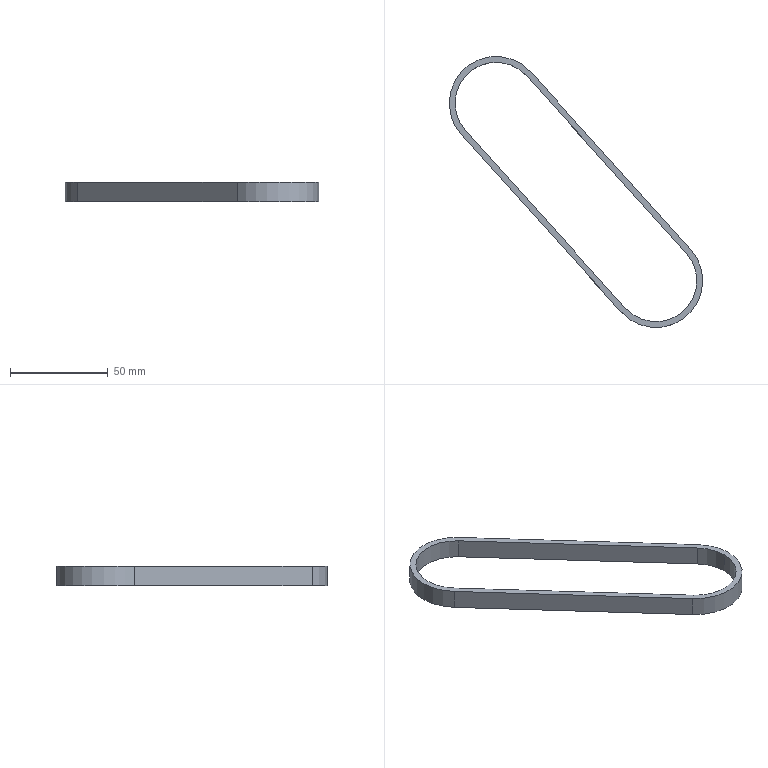Part | STEP file | 1 solid | 12 faces | box 130.012 x 138.996 x 10 mm | volume 11591 mm3 | plane 6 | cylinder 6 | commonest cylinder face diameters 42 x3 48 x3
STEP:
#1=CARTESIAN_POINT('',(0.,0.,0.));
#2=DIRECTION('',(0.,0.,1.));
#3=DIRECTION('',(1.,0.,0.));
#4=AXIS2_PLACEMENT_3D('',#1,#2,#3);
#5=CARTESIAN_POINT('',(-9.506,41.915,-2.));
#6=VERTEX_POINT('',#5);
#7=CARTESIAN_POINT('',(-91.518,132.912,-2.));
#8=VERTEX_POINT('',#7);
#9=CARTESIAN_POINT('',(15.599,14.059,-2.));
#10=DIRECTION('',(-0.6695,0.7428,0.));
#11=VECTOR('',#10,1.);
#12=LINE('',#9,#11);
#13=CARTESIAN_POINT('',(15.599,14.059,-12.));
#14=DIRECTION('',(0.7428,0.6695,0.));
#15=DIRECTION('',(0.,0.,-1.));
#16=AXIS2_PLACEMENT_3D('',#13,#14,#15);
#17=PLANE('',#16);
#18=CARTESIAN_POINT('',(-10.,0.));
#19=DIRECTION('',(0.,1.));
#20=VECTOR('',#19,1.);
#21=LINE('',#18,#20);
#22=(GEOMETRIC_REPRESENTATION_CONTEXT(2)PARAMETRIC_REPRESENTATION_CONTEXT()REPRESENTATION_CONTEXT('',''));
#23=DEFINITIONAL_REPRESENTATION('',(#21),#22);
#24=PCURVE('',#17,#23);
#25=CARTESIAN_POINT('',(0.,0.,-2.));
#26=DIRECTION('',(0.,0.,1.));
#27=DIRECTION('',(1.,0.,0.));
#28=AXIS2_PLACEMENT_3D('',#25,#26,#27);
#29=PLANE('',#28);
#30=CARTESIAN_POINT('',(15.599,14.059));
#31=DIRECTION('',(-0.6695,0.7428));
#32=VECTOR('',#31,1.);
#33=LINE('',#30,#32);
#34=(GEOMETRIC_REPRESENTATION_CONTEXT(2)PARAMETRIC_REPRESENTATION_CONTEXT()REPRESENTATION_CONTEXT('',''));
#35=DEFINITIONAL_REPRESENTATION('',(#33),#34);
#36=PCURVE('',#29,#35);
#37=SURFACE_CURVE('',#12,(#24,#36),.PCURVE_S1.);
#38=EDGE_CURVE('',#6,#8,#37,.T.);
#39=ORIENTED_EDGE('',*,*,#38,.T.);
#40=CARTESIAN_POINT('',(-91.518,132.912,-12.));
#41=VERTEX_POINT('',#40);
#42=CARTESIAN_POINT('',(-91.518,132.912,-12.));
#43=DIRECTION('',(0.,0.,1.));
#44=VECTOR('',#43,1.);
#45=LINE('',#42,#44);
#46=CARTESIAN_POINT('',(0.,160.));
#47=DIRECTION('',(-1.,0.));
#48=VECTOR('',#47,1.);
#49=LINE('',#46,#48);
#50=(GEOMETRIC_REPRESENTATION_CONTEXT(2)PARAMETRIC_REPRESENTATION_CONTEXT()REPRESENTATION_CONTEXT('',''));
#51=DEFINITIONAL_REPRESENTATION('',(#49),#50);
#52=PCURVE('',#17,#51);
#53=CARTESIAN_POINT('',(-107.117,118.852,-12.));
#54=DIRECTION('',(0.,0.,1.));
#55=DIRECTION('',(1.,0.,0.));
#56=AXIS2_PLACEMENT_3D('',#53,#54,#55);
#57=CYLINDRICAL_SURFACE('',#56,21.);
#58=CARTESIAN_POINT('',(0.7335,0.));
#59=DIRECTION('',(0.,1.));
#60=VECTOR('',#59,1.);
#61=LINE('',#58,#60);
#62=(GEOMETRIC_REPRESENTATION_CONTEXT(2)PARAMETRIC_REPRESENTATION_CONTEXT()REPRESENTATION_CONTEXT('',''));
#63=DEFINITIONAL_REPRESENTATION('',(#61),#62);
#64=PCURVE('',#57,#63);
#65=SURFACE_CURVE('',#45,(#52,#64),.PCURVE_S1.);
#66=EDGE_CURVE('',#41,#8,#65,.T.);
#67=ORIENTED_EDGE('',*,*,#66,.F.);
#68=CARTESIAN_POINT('',(-9.506,41.915,-12.));
#69=VERTEX_POINT('',#68);
#70=CARTESIAN_POINT('',(15.599,14.059,-12.));
#71=DIRECTION('',(-0.6695,0.7428,0.));
#72=VECTOR('',#71,1.);
#73=LINE('',#70,#72);
#74=CARTESIAN_POINT('',(0.,0.));
#75=DIRECTION('',(0.,1.));
#76=VECTOR('',#75,1.);
#77=LINE('',#74,#76);
#78=(GEOMETRIC_REPRESENTATION_CONTEXT(2)PARAMETRIC_REPRESENTATION_CONTEXT()REPRESENTATION_CONTEXT('',''));
#79=DEFINITIONAL_REPRESENTATION('',(#77),#78);
#80=PCURVE('',#17,#79);
#81=CARTESIAN_POINT('',(0.,0.,-12.));
#82=DIRECTION('',(0.,0.,1.));
#83=DIRECTION('',(1.,0.,0.));
#84=AXIS2_PLACEMENT_3D('',#81,#82,#83);
#85=PLANE('',#84);
#86=CARTESIAN_POINT('',(15.599,14.059));
#87=DIRECTION('',(-0.6695,0.7428));
#88=VECTOR('',#87,1.);
#89=LINE('',#86,#88);
#90=(GEOMETRIC_REPRESENTATION_CONTEXT(2)PARAMETRIC_REPRESENTATION_CONTEXT()REPRESENTATION_CONTEXT('',''));
#91=DEFINITIONAL_REPRESENTATION('',(#89),#90);
#92=PCURVE('',#85,#91);
#93=SURFACE_CURVE('',#73,(#80,#92),.PCURVE_S1.);
#94=EDGE_CURVE('',#69,#41,#93,.T.);
#95=ORIENTED_EDGE('',*,*,#94,.F.);
#96=CARTESIAN_POINT('',(-9.506,41.915,-12.));
#97=DIRECTION('',(0.,0.,1.));
#98=VECTOR('',#97,1.);
#99=LINE('',#96,#98);
#100=CARTESIAN_POINT('',(0.,37.5));
#101=DIRECTION('',(-1.,0.));
#102=VECTOR('',#101,1.);
#103=LINE('',#100,#102);
#104=(GEOMETRIC_REPRESENTATION_CONTEXT(2)PARAMETRIC_REPRESENTATION_CONTEXT()REPRESENTATION_CONTEXT('',''));
#105=DEFINITIONAL_REPRESENTATION('',(#103),#104);
#106=PCURVE('',#17,#105);
#107=CARTESIAN_POINT('',(-25.106,27.856,-12.));
#108=DIRECTION('',(0.,0.,1.));
#109=DIRECTION('',(1.,0.,0.));
#110=AXIS2_PLACEMENT_3D('',#107,#108,#109);
#111=CYLINDRICAL_SURFACE('',#110,21.);
#112=CARTESIAN_POINT('',(0.7335,0.));
#113=DIRECTION('',(0.,1.));
#114=VECTOR('',#113,1.);
#115=LINE('',#112,#114);
#116=(GEOMETRIC_REPRESENTATION_CONTEXT(2)PARAMETRIC_REPRESENTATION_CONTEXT()REPRESENTATION_CONTEXT('',''));
#117=DEFINITIONAL_REPRESENTATION('',(#115),#116);
#118=PCURVE('',#111,#117);
#119=SURFACE_CURVE('',#99,(#106,#118),.PCURVE_S1.);
#120=EDGE_CURVE('',#69,#6,#119,.T.);
#121=ORIENTED_EDGE('',*,*,#120,.T.);
#122=EDGE_LOOP('',(#39,#67,#95,#121));
#123=FACE_BOUND('',#122,.T.);
#124=ADVANCED_FACE('',(#123),#17,.F.);
#125=ORIENTED_EDGE('',*,*,#66,.F.);
#126=CARTESIAN_POINT('',(-122.717,104.793,-12.));
#127=VERTEX_POINT('',#126);
#128=CARTESIAN_POINT('',(-107.117,118.852,-12.));
#129=DIRECTION('',(0.,0.,1.));
#130=DIRECTION('',(1.,0.,0.));
#131=AXIS2_PLACEMENT_3D('',#128,#129,#130);
#132=CIRCLE('',#131,21.);
#133=CARTESIAN_POINT('',(0.,0.));
#134=DIRECTION('',(1.,0.));
#135=VECTOR('',#134,1.);
#136=LINE('',#133,#135);
#137=(GEOMETRIC_REPRESENTATION_CONTEXT(2)PARAMETRIC_REPRESENTATION_CONTEXT()REPRESENTATION_CONTEXT('',''));
#138=DEFINITIONAL_REPRESENTATION('',(#136),#137);
#139=PCURVE('',#57,#138);
#140=CARTESIAN_POINT('',(-107.117,118.852));
#141=DIRECTION('',(1.,0.));
#142=AXIS2_PLACEMENT_2D('',#140,#141);
#143=CIRCLE('',#142,21.);
#144=(GEOMETRIC_REPRESENTATION_CONTEXT(2)PARAMETRIC_REPRESENTATION_CONTEXT()REPRESENTATION_CONTEXT('',''));
#145=DEFINITIONAL_REPRESENTATION('',(#143),#144);
#146=PCURVE('',#85,#145);
#147=SURFACE_CURVE('',#132,(#139,#146),.PCURVE_S1.);
#148=EDGE_CURVE('',#41,#127,#147,.T.);
#149=ORIENTED_EDGE('',*,*,#148,.T.);
#150=CARTESIAN_POINT('',(-122.717,104.793,-2.));
#151=VERTEX_POINT('',#150);
#152=CARTESIAN_POINT('',(-122.717,104.793,-12.));
#153=DIRECTION('',(0.,0.,1.));
#154=VECTOR('',#153,1.);
#155=LINE('',#152,#154);
#156=CARTESIAN_POINT('',(3.875,0.));
#157=DIRECTION('',(0.,1.));
#158=VECTOR('',#157,1.);
#159=LINE('',#156,#158);
#160=(GEOMETRIC_REPRESENTATION_CONTEXT(2)PARAMETRIC_REPRESENTATION_CONTEXT()REPRESENTATION_CONTEXT('',''));
#161=DEFINITIONAL_REPRESENTATION('',(#159),#160);
#162=PCURVE('',#57,#161);
#163=CARTESIAN_POINT('',(-15.599,-14.059,-12.));
#164=DIRECTION('',(-0.7428,-0.6695,0.));
#165=DIRECTION('',(-0.6695,0.7428,0.));
#166=AXIS2_PLACEMENT_3D('',#163,#164,#165);
#167=PLANE('',#166);
#168=CARTESIAN_POINT('',(160.,0.));
#169=DIRECTION('',(0.,-1.));
#170=VECTOR('',#169,1.);
#171=LINE('',#168,#170);
#172=(GEOMETRIC_REPRESENTATION_CONTEXT(2)PARAMETRIC_REPRESENTATION_CONTEXT()REPRESENTATION_CONTEXT('',''));
#173=DEFINITIONAL_REPRESENTATION('',(#171),#172);
#174=PCURVE('',#167,#173);
#175=SURFACE_CURVE('',#155,(#162,#174),.PCURVE_S1.);
#176=EDGE_CURVE('',#127,#151,#175,.T.);
#177=ORIENTED_EDGE('',*,*,#176,.T.);
#178=CARTESIAN_POINT('',(-107.117,118.852,-2.));
#179=DIRECTION('',(0.,0.,1.));
#180=DIRECTION('',(1.,0.,0.));
#181=AXIS2_PLACEMENT_3D('',#178,#179,#180);
#182=CIRCLE('',#181,21.);
#183=CARTESIAN_POINT('',(0.,10.));
#184=DIRECTION('',(1.,0.));
#185=VECTOR('',#184,1.);
#186=LINE('',#183,#185);
#187=(GEOMETRIC_REPRESENTATION_CONTEXT(2)PARAMETRIC_REPRESENTATION_CONTEXT()REPRESENTATION_CONTEXT('',''));
#188=DEFINITIONAL_REPRESENTATION('',(#186),#187);
#189=PCURVE('',#57,#188);
#190=CARTESIAN_POINT('',(-107.117,118.852));
#191=DIRECTION('',(1.,0.));
#192=AXIS2_PLACEMENT_2D('',#190,#191);
#193=CIRCLE('',#192,21.);
#194=(GEOMETRIC_REPRESENTATION_CONTEXT(2)PARAMETRIC_REPRESENTATION_CONTEXT()REPRESENTATION_CONTEXT('',''));
#195=DEFINITIONAL_REPRESENTATION('',(#193),#194);
#196=PCURVE('',#29,#195);
#197=SURFACE_CURVE('',#182,(#189,#196),.PCURVE_S1.);
#198=EDGE_CURVE('',#8,#151,#197,.T.);
#199=ORIENTED_EDGE('',*,*,#198,.F.);
#200=EDGE_LOOP('',(#125,#149,#177,#199));
#201=FACE_BOUND('',#200,.F.);
#202=ADVANCED_FACE('',(#201),#57,.F.);
#203=CARTESIAN_POINT('',(-40.705,13.797,-2.));
#204=VERTEX_POINT('',#203);
#205=CARTESIAN_POINT('',(-15.599,-14.059,-2.));
#206=DIRECTION('',(0.6695,-0.7428,0.));
#207=VECTOR('',#206,1.);
#208=LINE('',#205,#207);
#209=CARTESIAN_POINT('',(0.,-10.));
#210=DIRECTION('',(-1.,0.));
#211=VECTOR('',#210,1.);
#212=LINE('',#209,#211);
#213=(GEOMETRIC_REPRESENTATION_CONTEXT(2)PARAMETRIC_REPRESENTATION_CONTEXT()REPRESENTATION_CONTEXT('',''));
#214=DEFINITIONAL_REPRESENTATION('',(#212),#213);
#215=PCURVE('',#167,#214);
#216=CARTESIAN_POINT('',(-15.599,-14.059));
#217=DIRECTION('',(0.6695,-0.7428));
#218=VECTOR('',#217,1.);
#219=LINE('',#216,#218);
#220=(GEOMETRIC_REPRESENTATION_CONTEXT(2)PARAMETRIC_REPRESENTATION_CONTEXT()REPRESENTATION_CONTEXT('',''));
#221=DEFINITIONAL_REPRESENTATION('',(#219),#220);
#222=PCURVE('',#29,#221);
#223=SURFACE_CURVE('',#208,(#215,#222),.PCURVE_S1.);
#224=EDGE_CURVE('',#151,#204,#223,.T.);
#225=ORIENTED_EDGE('',*,*,#224,.T.);
#226=CARTESIAN_POINT('',(-40.705,13.797,-12.));
#227=VERTEX_POINT('',#226);
#228=CARTESIAN_POINT('',(-40.705,13.797,-12.));
#229=DIRECTION('',(0.,0.,1.));
#230=VECTOR('',#229,1.);
#231=LINE('',#228,#230);
#232=CARTESIAN_POINT('',(37.5,0.));
#233=DIRECTION('',(0.,-1.));
#234=VECTOR('',#233,1.);
#235=LINE('',#232,#234);
#236=(GEOMETRIC_REPRESENTATION_CONTEXT(2)PARAMETRIC_REPRESENTATION_CONTEXT()REPRESENTATION_CONTEXT('',''));
#237=DEFINITIONAL_REPRESENTATION('',(#235),#236);
#238=PCURVE('',#167,#237);
#239=CARTESIAN_POINT('',(-25.106,27.856,-12.));
#240=DIRECTION('',(0.,0.,1.));
#241=DIRECTION('',(1.,0.,0.));
#242=AXIS2_PLACEMENT_3D('',#239,#240,#241);
#243=CYLINDRICAL_SURFACE('',#242,21.);
#244=CARTESIAN_POINT('',(3.875,0.));
#245=DIRECTION('',(0.,1.));
#246=VECTOR('',#245,1.);
#247=LINE('',#244,#246);
#248=(GEOMETRIC_REPRESENTATION_CONTEXT(2)PARAMETRIC_REPRESENTATION_CONTEXT()REPRESENTATION_CONTEXT('',''));
#249=DEFINITIONAL_REPRESENTATION('',(#247),#248);
#250=PCURVE('',#243,#249);
#251=SURFACE_CURVE('',#231,(#238,#250),.PCURVE_S1.);
#252=EDGE_CURVE('',#227,#204,#251,.T.);
#253=ORIENTED_EDGE('',*,*,#252,.F.);
#254=CARTESIAN_POINT('',(-15.599,-14.059,-12.));
#255=DIRECTION('',(0.6695,-0.7428,0.));
#256=VECTOR('',#255,1.);
#257=LINE('',#254,#256);
#258=CARTESIAN_POINT('',(0.,0.));
#259=DIRECTION('',(-1.,0.));
#260=VECTOR('',#259,1.);
#261=LINE('',#258,#260);
#262=(GEOMETRIC_REPRESENTATION_CONTEXT(2)PARAMETRIC_REPRESENTATION_CONTEXT()REPRESENTATION_CONTEXT('',''));
#263=DEFINITIONAL_REPRESENTATION('',(#261),#262);
#264=PCURVE('',#167,#263);
#265=CARTESIAN_POINT('',(-15.599,-14.059));
#266=DIRECTION('',(0.6695,-0.7428));
#267=VECTOR('',#266,1.);
#268=LINE('',#265,#267);
#269=(GEOMETRIC_REPRESENTATION_CONTEXT(2)PARAMETRIC_REPRESENTATION_CONTEXT()REPRESENTATION_CONTEXT('',''));
#270=DEFINITIONAL_REPRESENTATION('',(#268),#269);
#271=PCURVE('',#85,#270);
#272=SURFACE_CURVE('',#257,(#264,#271),.PCURVE_S1.);
#273=EDGE_CURVE('',#127,#227,#272,.T.);
#274=ORIENTED_EDGE('',*,*,#273,.F.);
#275=ORIENTED_EDGE('',*,*,#176,.T.);
#276=EDGE_LOOP('',(#225,#253,#274,#275));
#277=FACE_BOUND('',#276,.T.);
#278=ADVANCED_FACE('',(#277),#167,.F.);
#279=CARTESIAN_POINT('',(-4.106,27.856,-2.));
#280=VERTEX_POINT('',#279);
#281=CARTESIAN_POINT('',(-25.106,27.856,-2.));
#282=DIRECTION('',(0.,0.,1.));
#283=DIRECTION('',(1.,0.,0.));
#284=AXIS2_PLACEMENT_3D('',#281,#282,#283);
#285=CIRCLE('',#284,21.);
#286=CARTESIAN_POINT('',(0.,10.));
#287=DIRECTION('',(1.,0.));
#288=VECTOR('',#287,1.);
#289=LINE('',#286,#288);
#290=(GEOMETRIC_REPRESENTATION_CONTEXT(2)PARAMETRIC_REPRESENTATION_CONTEXT()REPRESENTATION_CONTEXT('',''));
#291=DEFINITIONAL_REPRESENTATION('',(#289),#290);
#292=PCURVE('',#243,#291);
#293=CARTESIAN_POINT('',(-25.106,27.856));
#294=DIRECTION('',(1.,0.));
#295=AXIS2_PLACEMENT_2D('',#293,#294);
#296=CIRCLE('',#295,21.);
#297=(GEOMETRIC_REPRESENTATION_CONTEXT(2)PARAMETRIC_REPRESENTATION_CONTEXT()REPRESENTATION_CONTEXT('',''));
#298=DEFINITIONAL_REPRESENTATION('',(#296),#297);
#299=PCURVE('',#29,#298);
#300=SURFACE_CURVE('',#285,(#292,#299),.PCURVE_S1.);
#301=EDGE_CURVE('',#204,#280,#300,.T.);
#302=ORIENTED_EDGE('',*,*,#301,.F.);
#303=ORIENTED_EDGE('',*,*,#252,.F.);
#304=CARTESIAN_POINT('',(-4.106,27.856,-12.));
#305=VERTEX_POINT('',#304);
#306=CARTESIAN_POINT('',(-25.106,27.856,-12.));
#307=DIRECTION('',(0.,0.,1.));
#308=DIRECTION('',(1.,0.,0.));
#309=AXIS2_PLACEMENT_3D('',#306,#307,#308);
#310=CIRCLE('',#309,21.);
#311=CARTESIAN_POINT('',(0.,0.));
#312=DIRECTION('',(1.,0.));
#313=VECTOR('',#312,1.);
#314=LINE('',#311,#313);
#315=(GEOMETRIC_REPRESENTATION_CONTEXT(2)PARAMETRIC_REPRESENTATION_CONTEXT()REPRESENTATION_CONTEXT('',''));
#316=DEFINITIONAL_REPRESENTATION('',(#314),#315);
#317=PCURVE('',#243,#316);
#318=CARTESIAN_POINT('',(-25.106,27.856));
#319=DIRECTION('',(1.,0.));
#320=AXIS2_PLACEMENT_2D('',#318,#319);
#321=CIRCLE('',#320,21.);
#322=(GEOMETRIC_REPRESENTATION_CONTEXT(2)PARAMETRIC_REPRESENTATION_CONTEXT()REPRESENTATION_CONTEXT('',''));
#323=DEFINITIONAL_REPRESENTATION('',(#321),#322);
#324=PCURVE('',#85,#323);
#325=SURFACE_CURVE('',#310,(#317,#324),.PCURVE_S1.);
#326=EDGE_CURVE('',#227,#305,#325,.T.);
#327=ORIENTED_EDGE('',*,*,#326,.T.);
#328=CARTESIAN_POINT('',(-4.106,27.856,-12.));
#329=DIRECTION('',(0.,0.,1.));
#330=VECTOR('',#329,1.);
#331=LINE('',#328,#330);
#332=CARTESIAN_POINT('',(6.283,0.));
#333=DIRECTION('',(0.,1.));
#334=VECTOR('',#333,1.);
#335=LINE('',#332,#334);
#336=(GEOMETRIC_REPRESENTATION_CONTEXT(2)PARAMETRIC_REPRESENTATION_CONTEXT()REPRESENTATION_CONTEXT('',''));
#337=DEFINITIONAL_REPRESENTATION('',(#335),#336);
#338=PCURVE('',#243,#337);
#339=CARTESIAN_POINT('',(0.,0.));
#340=DIRECTION('',(0.,1.));
#341=VECTOR('',#340,1.);
#342=LINE('',#339,#341);
#343=(GEOMETRIC_REPRESENTATION_CONTEXT(2)PARAMETRIC_REPRESENTATION_CONTEXT()REPRESENTATION_CONTEXT('',''));
#344=DEFINITIONAL_REPRESENTATION('',(#342),#343);
#345=PCURVE('',#111,#344);
#346=SURFACE_CURVE('',#331,(#338,#345),.PCURVE_S1.);
#347=EDGE_CURVE('',#305,#280,#346,.T.);
#348=ORIENTED_EDGE('',*,*,#347,.T.);
#349=EDGE_LOOP('',(#302,#303,#327,#348));
#350=FACE_BOUND('',#349,.F.);
#351=ADVANCED_FACE('',(#350),#243,.F.);
#352=ORIENTED_EDGE('',*,*,#301,.F.);
#353=ORIENTED_EDGE('',*,*,#224,.F.);
#354=ORIENTED_EDGE('',*,*,#198,.F.);
#355=ORIENTED_EDGE('',*,*,#38,.F.);
#356=CARTESIAN_POINT('',(-25.106,27.856,-2.));
#357=DIRECTION('',(0.,0.,1.));
#358=DIRECTION('',(1.,0.,0.));
#359=AXIS2_PLACEMENT_3D('',#356,#357,#358);
#360=CIRCLE('',#359,21.);
#361=CARTESIAN_POINT('',(-25.106,27.856));
#362=DIRECTION('',(1.,0.));
#363=AXIS2_PLACEMENT_2D('',#361,#362);
#364=CIRCLE('',#363,21.);
#365=(GEOMETRIC_REPRESENTATION_CONTEXT(2)PARAMETRIC_REPRESENTATION_CONTEXT()REPRESENTATION_CONTEXT('',''));
#366=DEFINITIONAL_REPRESENTATION('',(#364),#365);
#367=PCURVE('',#29,#366);
#368=CARTESIAN_POINT('',(0.,10.));
#369=DIRECTION('',(1.,0.));
#370=VECTOR('',#369,1.);
#371=LINE('',#368,#370);
#372=(GEOMETRIC_REPRESENTATION_CONTEXT(2)PARAMETRIC_REPRESENTATION_CONTEXT()REPRESENTATION_CONTEXT('',''));
#373=DEFINITIONAL_REPRESENTATION('',(#371),#372);
#374=PCURVE('',#111,#373);
#375=SURFACE_CURVE('',#360,(#367,#374),.PCURVE_S1.);
#376=EDGE_CURVE('',#280,#6,#375,.T.);
#377=ORIENTED_EDGE('',*,*,#376,.F.);
#378=EDGE_LOOP('',(#352,#353,#354,#355,#377));
#379=FACE_BOUND('',#378,.T.);
#380=CARTESIAN_POINT('',(-42.933,11.788,-2.));
#381=VERTEX_POINT('',#380);
#382=CARTESIAN_POINT('',(-1.106,27.856,-2.));
#383=VERTEX_POINT('',#382);
#384=CARTESIAN_POINT('',(-25.106,27.856,-2.));
#385=DIRECTION('',(0.,0.,1.));
#386=DIRECTION('',(1.,0.,0.));
#387=AXIS2_PLACEMENT_3D('',#384,#385,#386);
#388=CIRCLE('',#387,24.);
#389=CARTESIAN_POINT('',(-25.106,27.856));
#390=DIRECTION('',(1.,0.));
#391=AXIS2_PLACEMENT_2D('',#389,#390);
#392=CIRCLE('',#391,24.);
#393=(GEOMETRIC_REPRESENTATION_CONTEXT(2)PARAMETRIC_REPRESENTATION_CONTEXT()REPRESENTATION_CONTEXT('',''));
#394=DEFINITIONAL_REPRESENTATION('',(#392),#393);
#395=PCURVE('',#29,#394);
#396=CARTESIAN_POINT('',(-25.106,27.856,-12.));
#397=DIRECTION('',(0.,0.,1.));
#398=DIRECTION('',(1.,0.,0.));
#399=AXIS2_PLACEMENT_3D('',#396,#397,#398);
#400=CYLINDRICAL_SURFACE('',#399,24.);
#401=CARTESIAN_POINT('',(0.,10.));
#402=DIRECTION('',(1.,0.));
#403=VECTOR('',#402,1.);
#404=LINE('',#401,#403);
#405=(GEOMETRIC_REPRESENTATION_CONTEXT(2)PARAMETRIC_REPRESENTATION_CONTEXT()REPRESENTATION_CONTEXT('',''));
#406=DEFINITIONAL_REPRESENTATION('',(#404),#405);
#407=PCURVE('',#400,#406);
#408=SURFACE_CURVE('',#388,(#395,#407),.PCURVE_S1.);
#409=EDGE_CURVE('',#381,#383,#408,.T.);
#410=ORIENTED_EDGE('',*,*,#409,.T.);
#411=CARTESIAN_POINT('',(-7.278,43.924,-2.));
#412=VERTEX_POINT('',#411);
#413=CARTESIAN_POINT('',(-25.106,27.856,-2.));
#414=DIRECTION('',(0.,0.,1.));
#415=DIRECTION('',(1.,0.,0.));
#416=AXIS2_PLACEMENT_3D('',#413,#414,#415);
#417=CIRCLE('',#416,24.);
#418=CARTESIAN_POINT('',(-25.106,27.856));
#419=DIRECTION('',(1.,0.));
#420=AXIS2_PLACEMENT_2D('',#418,#419);
#421=CIRCLE('',#420,24.);
#422=(GEOMETRIC_REPRESENTATION_CONTEXT(2)PARAMETRIC_REPRESENTATION_CONTEXT()REPRESENTATION_CONTEXT('',''));
#423=DEFINITIONAL_REPRESENTATION('',(#421),#422);
#424=PCURVE('',#29,#423);
#425=CARTESIAN_POINT('',(-25.106,27.856,-12.));
#426=DIRECTION('',(0.,0.,1.));
#427=DIRECTION('',(1.,0.,0.));
#428=AXIS2_PLACEMENT_3D('',#425,#426,#427);
#429=CYLINDRICAL_SURFACE('',#428,24.);
#430=CARTESIAN_POINT('',(0.,10.));
#431=DIRECTION('',(1.,0.));
#432=VECTOR('',#431,1.);
#433=LINE('',#430,#432);
#434=(GEOMETRIC_REPRESENTATION_CONTEXT(2)PARAMETRIC_REPRESENTATION_CONTEXT()REPRESENTATION_CONTEXT('',''));
#435=DEFINITIONAL_REPRESENTATION('',(#433),#434);
#436=PCURVE('',#429,#435);
#437=SURFACE_CURVE('',#417,(#424,#436),.PCURVE_S1.);
#438=EDGE_CURVE('',#383,#412,#437,.T.);
#439=ORIENTED_EDGE('',*,*,#438,.T.);
#440=CARTESIAN_POINT('',(-89.289,134.92,-2.));
#441=VERTEX_POINT('',#440);
#442=CARTESIAN_POINT('',(17.828,16.068,-2.));
#443=DIRECTION('',(-0.6695,0.7428,0.));
#444=VECTOR('',#443,1.);
#445=LINE('',#442,#444);
#446=CARTESIAN_POINT('',(17.828,16.068));
#447=DIRECTION('',(-0.6695,0.7428));
#448=VECTOR('',#447,1.);
#449=LINE('',#446,#448);
#450=(GEOMETRIC_REPRESENTATION_CONTEXT(2)PARAMETRIC_REPRESENTATION_CONTEXT()REPRESENTATION_CONTEXT('',''));
#451=DEFINITIONAL_REPRESENTATION('',(#449),#450);
#452=PCURVE('',#29,#451);
#453=CARTESIAN_POINT('',(17.828,16.068,-12.));
#454=DIRECTION('',(0.7428,0.6695,0.));
#455=DIRECTION('',(0.,0.,-1.));
#456=AXIS2_PLACEMENT_3D('',#453,#454,#455);
#457=PLANE('',#456);
#458=CARTESIAN_POINT('',(-10.,0.));
#459=DIRECTION('',(0.,1.));
#460=VECTOR('',#459,1.);
#461=LINE('',#458,#460);
#462=(GEOMETRIC_REPRESENTATION_CONTEXT(2)PARAMETRIC_REPRESENTATION_CONTEXT()REPRESENTATION_CONTEXT('',''));
#463=DEFINITIONAL_REPRESENTATION('',(#461),#462);
#464=PCURVE('',#457,#463);
#465=SURFACE_CURVE('',#445,(#452,#464),.PCURVE_S1.);
#466=EDGE_CURVE('',#412,#441,#465,.T.);
#467=ORIENTED_EDGE('',*,*,#466,.T.);
#468=CARTESIAN_POINT('',(-124.945,102.785,-2.));
#469=VERTEX_POINT('',#468);
#470=CARTESIAN_POINT('',(-107.117,118.852,-2.));
#471=DIRECTION('',(0.,0.,1.));
#472=DIRECTION('',(1.,0.,0.));
#473=AXIS2_PLACEMENT_3D('',#470,#471,#472);
#474=CIRCLE('',#473,24.);
#475=CARTESIAN_POINT('',(-107.117,118.852));
#476=DIRECTION('',(1.,0.));
#477=AXIS2_PLACEMENT_2D('',#475,#476);
#478=CIRCLE('',#477,24.);
#479=(GEOMETRIC_REPRESENTATION_CONTEXT(2)PARAMETRIC_REPRESENTATION_CONTEXT()REPRESENTATION_CONTEXT('',''));
#480=DEFINITIONAL_REPRESENTATION('',(#478),#479);
#481=PCURVE('',#29,#480);
#482=CARTESIAN_POINT('',(-107.117,118.852,-12.));
#483=DIRECTION('',(0.,0.,1.));
#484=DIRECTION('',(1.,0.,0.));
#485=AXIS2_PLACEMENT_3D('',#482,#483,#484);
#486=CYLINDRICAL_SURFACE('',#485,24.);
#487=CARTESIAN_POINT('',(0.,10.));
#488=DIRECTION('',(1.,0.));
#489=VECTOR('',#488,1.);
#490=LINE('',#487,#489);
#491=(GEOMETRIC_REPRESENTATION_CONTEXT(2)PARAMETRIC_REPRESENTATION_CONTEXT()REPRESENTATION_CONTEXT('',''));
#492=DEFINITIONAL_REPRESENTATION('',(#490),#491);
#493=PCURVE('',#486,#492);
#494=SURFACE_CURVE('',#474,(#481,#493),.PCURVE_S1.);
#495=EDGE_CURVE('',#441,#469,#494,.T.);
#496=ORIENTED_EDGE('',*,*,#495,.T.);
#497=CARTESIAN_POINT('',(-17.828,-16.068,-2.));
#498=DIRECTION('',(0.6695,-0.7428,0.));
#499=VECTOR('',#498,1.);
#500=LINE('',#497,#499);
#501=CARTESIAN_POINT('',(-17.828,-16.068));
#502=DIRECTION('',(0.6695,-0.7428));
#503=VECTOR('',#502,1.);
#504=LINE('',#501,#503);
#505=(GEOMETRIC_REPRESENTATION_CONTEXT(2)PARAMETRIC_REPRESENTATION_CONTEXT()REPRESENTATION_CONTEXT('',''));
#506=DEFINITIONAL_REPRESENTATION('',(#504),#505);
#507=PCURVE('',#29,#506);
#508=CARTESIAN_POINT('',(-17.828,-16.068,-12.));
#509=DIRECTION('',(-0.7428,-0.6695,0.));
#510=DIRECTION('',(-0.6695,0.7428,0.));
#511=AXIS2_PLACEMENT_3D('',#508,#509,#510);
#512=PLANE('',#511);
#513=CARTESIAN_POINT('',(0.,-10.));
#514=DIRECTION('',(-1.,0.));
#515=VECTOR('',#514,1.);
#516=LINE('',#513,#515);
#517=(GEOMETRIC_REPRESENTATION_CONTEXT(2)PARAMETRIC_REPRESENTATION_CONTEXT()REPRESENTATION_CONTEXT('',''));
#518=DEFINITIONAL_REPRESENTATION('',(#516),#517);
#519=PCURVE('',#512,#518);
#520=SURFACE_CURVE('',#500,(#507,#519),.PCURVE_S1.);
#521=EDGE_CURVE('',#469,#381,#520,.T.);
#522=ORIENTED_EDGE('',*,*,#521,.T.);
#523=EDGE_LOOP('',(#410,#439,#467,#496,#522));
#524=FACE_BOUND('',#523,.T.);
#525=ADVANCED_FACE('',(#379,#524),#29,.T.);
#526=ORIENTED_EDGE('',*,*,#273,.T.);
#527=ORIENTED_EDGE('',*,*,#326,.T.);
#528=CARTESIAN_POINT('',(-25.106,27.856,-12.));
#529=DIRECTION('',(0.,0.,1.));
#530=DIRECTION('',(1.,0.,0.));
#531=AXIS2_PLACEMENT_3D('',#528,#529,#530);
#532=CIRCLE('',#531,21.);
#533=CARTESIAN_POINT('',(-25.106,27.856));
#534=DIRECTION('',(1.,0.));
#535=AXIS2_PLACEMENT_2D('',#533,#534);
#536=CIRCLE('',#535,21.);
#537=(GEOMETRIC_REPRESENTATION_CONTEXT(2)PARAMETRIC_REPRESENTATION_CONTEXT()REPRESENTATION_CONTEXT('',''));
#538=DEFINITIONAL_REPRESENTATION('',(#536),#537);
#539=PCURVE('',#85,#538);
#540=CARTESIAN_POINT('',(0.,0.));
#541=DIRECTION('',(1.,0.));
#542=VECTOR('',#541,1.);
#543=LINE('',#540,#542);
#544=(GEOMETRIC_REPRESENTATION_CONTEXT(2)PARAMETRIC_REPRESENTATION_CONTEXT()REPRESENTATION_CONTEXT('',''));
#545=DEFINITIONAL_REPRESENTATION('',(#543),#544);
#546=PCURVE('',#111,#545);
#547=SURFACE_CURVE('',#532,(#539,#546),.PCURVE_S1.);
#548=EDGE_CURVE('',#305,#69,#547,.T.);
#549=ORIENTED_EDGE('',*,*,#548,.T.);
#550=ORIENTED_EDGE('',*,*,#94,.T.);
#551=ORIENTED_EDGE('',*,*,#148,.T.);
#552=EDGE_LOOP('',(#526,#527,#549,#550,#551));
#553=FACE_BOUND('',#552,.T.);
#554=CARTESIAN_POINT('',(-42.933,11.788,-12.));
#555=VERTEX_POINT('',#554);
#556=CARTESIAN_POINT('',(-1.106,27.856,-12.));
#557=VERTEX_POINT('',#556);
#558=CARTESIAN_POINT('',(-25.106,27.856,-12.));
#559=DIRECTION('',(0.,0.,1.));
#560=DIRECTION('',(1.,0.,0.));
#561=AXIS2_PLACEMENT_3D('',#558,#559,#560);
#562=CIRCLE('',#561,24.);
#563=CARTESIAN_POINT('',(-25.106,27.856));
#564=DIRECTION('',(1.,0.));
#565=AXIS2_PLACEMENT_2D('',#563,#564);
#566=CIRCLE('',#565,24.);
#567=(GEOMETRIC_REPRESENTATION_CONTEXT(2)PARAMETRIC_REPRESENTATION_CONTEXT()REPRESENTATION_CONTEXT('',''));
#568=DEFINITIONAL_REPRESENTATION('',(#566),#567);
#569=PCURVE('',#85,#568);
#570=CARTESIAN_POINT('',(0.,0.));
#571=DIRECTION('',(1.,0.));
#572=VECTOR('',#571,1.);
#573=LINE('',#570,#572);
#574=(GEOMETRIC_REPRESENTATION_CONTEXT(2)PARAMETRIC_REPRESENTATION_CONTEXT()REPRESENTATION_CONTEXT('',''));
#575=DEFINITIONAL_REPRESENTATION('',(#573),#574);
#576=PCURVE('',#400,#575);
#577=SURFACE_CURVE('',#562,(#569,#576),.PCURVE_S1.);
#578=EDGE_CURVE('',#555,#557,#577,.T.);
#579=ORIENTED_EDGE('',*,*,#578,.F.);
#580=CARTESIAN_POINT('',(-124.945,102.785,-12.));
#581=VERTEX_POINT('',#580);
#582=CARTESIAN_POINT('',(-17.828,-16.068,-12.));
#583=DIRECTION('',(0.6695,-0.7428,0.));
#584=VECTOR('',#583,1.);
#585=LINE('',#582,#584);
#586=CARTESIAN_POINT('',(-17.828,-16.068));
#587=DIRECTION('',(0.6695,-0.7428));
#588=VECTOR('',#587,1.);
#589=LINE('',#586,#588);
#590=(GEOMETRIC_REPRESENTATION_CONTEXT(2)PARAMETRIC_REPRESENTATION_CONTEXT()REPRESENTATION_CONTEXT('',''));
#591=DEFINITIONAL_REPRESENTATION('',(#589),#590);
#592=PCURVE('',#85,#591);
#593=CARTESIAN_POINT('',(0.,0.));
#594=DIRECTION('',(-1.,0.));
#595=VECTOR('',#594,1.);
#596=LINE('',#593,#595);
#597=(GEOMETRIC_REPRESENTATION_CONTEXT(2)PARAMETRIC_REPRESENTATION_CONTEXT()REPRESENTATION_CONTEXT('',''));
#598=DEFINITIONAL_REPRESENTATION('',(#596),#597);
#599=PCURVE('',#512,#598);
#600=SURFACE_CURVE('',#585,(#592,#599),.PCURVE_S1.);
#601=EDGE_CURVE('',#581,#555,#600,.T.);
#602=ORIENTED_EDGE('',*,*,#601,.F.);
#603=CARTESIAN_POINT('',(-89.289,134.92,-12.));
#604=VERTEX_POINT('',#603);
#605=CARTESIAN_POINT('',(-107.117,118.852,-12.));
#606=DIRECTION('',(0.,0.,1.));
#607=DIRECTION('',(1.,0.,0.));
#608=AXIS2_PLACEMENT_3D('',#605,#606,#607);
#609=CIRCLE('',#608,24.);
#610=CARTESIAN_POINT('',(-107.117,118.852));
#611=DIRECTION('',(1.,0.));
#612=AXIS2_PLACEMENT_2D('',#610,#611);
#613=CIRCLE('',#612,24.);
#614=(GEOMETRIC_REPRESENTATION_CONTEXT(2)PARAMETRIC_REPRESENTATION_CONTEXT()REPRESENTATION_CONTEXT('',''));
#615=DEFINITIONAL_REPRESENTATION('',(#613),#614);
#616=PCURVE('',#85,#615);
#617=CARTESIAN_POINT('',(0.,0.));
#618=DIRECTION('',(1.,0.));
#619=VECTOR('',#618,1.);
#620=LINE('',#617,#619);
#621=(GEOMETRIC_REPRESENTATION_CONTEXT(2)PARAMETRIC_REPRESENTATION_CONTEXT()REPRESENTATION_CONTEXT('',''));
#622=DEFINITIONAL_REPRESENTATION('',(#620),#621);
#623=PCURVE('',#486,#622);
#624=SURFACE_CURVE('',#609,(#616,#623),.PCURVE_S1.);
#625=EDGE_CURVE('',#604,#581,#624,.T.);
#626=ORIENTED_EDGE('',*,*,#625,.F.);
#627=CARTESIAN_POINT('',(-7.278,43.924,-12.));
#628=VERTEX_POINT('',#627);
#629=CARTESIAN_POINT('',(17.828,16.068,-12.));
#630=DIRECTION('',(-0.6695,0.7428,0.));
#631=VECTOR('',#630,1.);
#632=LINE('',#629,#631);
#633=CARTESIAN_POINT('',(17.828,16.068));
#634=DIRECTION('',(-0.6695,0.7428));
#635=VECTOR('',#634,1.);
#636=LINE('',#633,#635);
#637=(GEOMETRIC_REPRESENTATION_CONTEXT(2)PARAMETRIC_REPRESENTATION_CONTEXT()REPRESENTATION_CONTEXT('',''));
#638=DEFINITIONAL_REPRESENTATION('',(#636),#637);
#639=PCURVE('',#85,#638);
#640=CARTESIAN_POINT('',(0.,0.));
#641=DIRECTION('',(0.,1.));
#642=VECTOR('',#641,1.);
#643=LINE('',#640,#642);
#644=(GEOMETRIC_REPRESENTATION_CONTEXT(2)PARAMETRIC_REPRESENTATION_CONTEXT()REPRESENTATION_CONTEXT('',''));
#645=DEFINITIONAL_REPRESENTATION('',(#643),#644);
#646=PCURVE('',#457,#645);
#647=SURFACE_CURVE('',#632,(#639,#646),.PCURVE_S1.);
#648=EDGE_CURVE('',#628,#604,#647,.T.);
#649=ORIENTED_EDGE('',*,*,#648,.F.);
#650=CARTESIAN_POINT('',(-25.106,27.856,-12.));
#651=DIRECTION('',(0.,0.,1.));
#652=DIRECTION('',(1.,0.,0.));
#653=AXIS2_PLACEMENT_3D('',#650,#651,#652);
#654=CIRCLE('',#653,24.);
#655=CARTESIAN_POINT('',(-25.106,27.856));
#656=DIRECTION('',(1.,0.));
#657=AXIS2_PLACEMENT_2D('',#655,#656);
#658=CIRCLE('',#657,24.);
#659=(GEOMETRIC_REPRESENTATION_CONTEXT(2)PARAMETRIC_REPRESENTATION_CONTEXT()REPRESENTATION_CONTEXT('',''));
#660=DEFINITIONAL_REPRESENTATION('',(#658),#659);
#661=PCURVE('',#85,#660);
#662=CARTESIAN_POINT('',(0.,0.));
#663=DIRECTION('',(1.,0.));
#664=VECTOR('',#663,1.);
#665=LINE('',#662,#664);
#666=(GEOMETRIC_REPRESENTATION_CONTEXT(2)PARAMETRIC_REPRESENTATION_CONTEXT()REPRESENTATION_CONTEXT('',''));
#667=DEFINITIONAL_REPRESENTATION('',(#665),#666);
#668=PCURVE('',#429,#667);
#669=SURFACE_CURVE('',#654,(#661,#668),.PCURVE_S1.);
#670=EDGE_CURVE('',#557,#628,#669,.T.);
#671=ORIENTED_EDGE('',*,*,#670,.F.);
#672=EDGE_LOOP('',(#579,#602,#626,#649,#671));
#673=FACE_BOUND('',#672,.T.);
#674=ADVANCED_FACE('',(#553,#673),#85,.F.);
#675=ORIENTED_EDGE('',*,*,#466,.F.);
#676=CARTESIAN_POINT('',(-7.278,43.924,-12.));
#677=DIRECTION('',(0.,0.,1.));
#678=VECTOR('',#677,1.);
#679=LINE('',#676,#678);
#680=CARTESIAN_POINT('',(0.,37.5));
#681=DIRECTION('',(-1.,0.));
#682=VECTOR('',#681,1.);
#683=LINE('',#680,#682);
#684=(GEOMETRIC_REPRESENTATION_CONTEXT(2)PARAMETRIC_REPRESENTATION_CONTEXT()REPRESENTATION_CONTEXT('',''));
#685=DEFINITIONAL_REPRESENTATION('',(#683),#684);
#686=PCURVE('',#457,#685);
#687=CARTESIAN_POINT('',(0.7335,0.));
#688=DIRECTION('',(0.,1.));
#689=VECTOR('',#688,1.);
#690=LINE('',#687,#689);
#691=(GEOMETRIC_REPRESENTATION_CONTEXT(2)PARAMETRIC_REPRESENTATION_CONTEXT()REPRESENTATION_CONTEXT('',''));
#692=DEFINITIONAL_REPRESENTATION('',(#690),#691);
#693=PCURVE('',#429,#692);
#694=SURFACE_CURVE('',#679,(#686,#693),.PCURVE_S1.);
#695=EDGE_CURVE('',#628,#412,#694,.T.);
#696=ORIENTED_EDGE('',*,*,#695,.F.);
#697=ORIENTED_EDGE('',*,*,#648,.T.);
#698=CARTESIAN_POINT('',(-89.289,134.92,-12.));
#699=DIRECTION('',(0.,0.,1.));
#700=VECTOR('',#699,1.);
#701=LINE('',#698,#700);
#702=CARTESIAN_POINT('',(0.,160.));
#703=DIRECTION('',(-1.,0.));
#704=VECTOR('',#703,1.);
#705=LINE('',#702,#704);
#706=(GEOMETRIC_REPRESENTATION_CONTEXT(2)PARAMETRIC_REPRESENTATION_CONTEXT()REPRESENTATION_CONTEXT('',''));
#707=DEFINITIONAL_REPRESENTATION('',(#705),#706);
#708=PCURVE('',#457,#707);
#709=CARTESIAN_POINT('',(0.7335,0.));
#710=DIRECTION('',(0.,1.));
#711=VECTOR('',#710,1.);
#712=LINE('',#709,#711);
#713=(GEOMETRIC_REPRESENTATION_CONTEXT(2)PARAMETRIC_REPRESENTATION_CONTEXT()REPRESENTATION_CONTEXT('',''));
#714=DEFINITIONAL_REPRESENTATION('',(#712),#713);
#715=PCURVE('',#486,#714);
#716=SURFACE_CURVE('',#701,(#708,#715),.PCURVE_S1.);
#717=EDGE_CURVE('',#604,#441,#716,.T.);
#718=ORIENTED_EDGE('',*,*,#717,.T.);
#719=EDGE_LOOP('',(#675,#696,#697,#718));
#720=FACE_BOUND('',#719,.T.);
#721=ADVANCED_FACE('',(#720),#457,.T.);
#722=ORIENTED_EDGE('',*,*,#495,.F.);
#723=ORIENTED_EDGE('',*,*,#717,.F.);
#724=ORIENTED_EDGE('',*,*,#625,.T.);
#725=CARTESIAN_POINT('',(-124.945,102.785,-12.));
#726=DIRECTION('',(0.,0.,1.));
#727=VECTOR('',#726,1.);
#728=LINE('',#725,#727);
#729=CARTESIAN_POINT('',(3.875,0.));
#730=DIRECTION('',(0.,1.));
#731=VECTOR('',#730,1.);
#732=LINE('',#729,#731);
#733=(GEOMETRIC_REPRESENTATION_CONTEXT(2)PARAMETRIC_REPRESENTATION_CONTEXT()REPRESENTATION_CONTEXT('',''));
#734=DEFINITIONAL_REPRESENTATION('',(#732),#733);
#735=PCURVE('',#486,#734);
#736=CARTESIAN_POINT('',(160.,0.));
#737=DIRECTION('',(0.,-1.));
#738=VECTOR('',#737,1.);
#739=LINE('',#736,#738);
#740=(GEOMETRIC_REPRESENTATION_CONTEXT(2)PARAMETRIC_REPRESENTATION_CONTEXT()REPRESENTATION_CONTEXT('',''));
#741=DEFINITIONAL_REPRESENTATION('',(#739),#740);
#742=PCURVE('',#512,#741);
#743=SURFACE_CURVE('',#728,(#735,#742),.PCURVE_S1.);
#744=EDGE_CURVE('',#581,#469,#743,.T.);
#745=ORIENTED_EDGE('',*,*,#744,.T.);
#746=EDGE_LOOP('',(#722,#723,#724,#745));
#747=FACE_BOUND('',#746,.T.);
#748=ADVANCED_FACE('',(#747),#486,.T.);
#749=ORIENTED_EDGE('',*,*,#521,.F.);
#750=ORIENTED_EDGE('',*,*,#744,.F.);
#751=ORIENTED_EDGE('',*,*,#601,.T.);
#752=CARTESIAN_POINT('',(-42.933,11.788,-12.));
#753=DIRECTION('',(0.,0.,1.));
#754=VECTOR('',#753,1.);
#755=LINE('',#752,#754);
#756=CARTESIAN_POINT('',(37.5,0.));
#757=DIRECTION('',(0.,-1.));
#758=VECTOR('',#757,1.);
#759=LINE('',#756,#758);
#760=(GEOMETRIC_REPRESENTATION_CONTEXT(2)PARAMETRIC_REPRESENTATION_CONTEXT()REPRESENTATION_CONTEXT('',''));
#761=DEFINITIONAL_REPRESENTATION('',(#759),#760);
#762=PCURVE('',#512,#761);
#763=CARTESIAN_POINT('',(3.875,0.));
#764=DIRECTION('',(0.,1.));
#765=VECTOR('',#764,1.);
#766=LINE('',#763,#765);
#767=(GEOMETRIC_REPRESENTATION_CONTEXT(2)PARAMETRIC_REPRESENTATION_CONTEXT()REPRESENTATION_CONTEXT('',''));
#768=DEFINITIONAL_REPRESENTATION('',(#766),#767);
#769=PCURVE('',#400,#768);
#770=SURFACE_CURVE('',#755,(#762,#769),.PCURVE_S1.);
#771=EDGE_CURVE('',#555,#381,#770,.T.);
#772=ORIENTED_EDGE('',*,*,#771,.T.);
#773=EDGE_LOOP('',(#749,#750,#751,#772));
#774=FACE_BOUND('',#773,.T.);
#775=ADVANCED_FACE('',(#774),#512,.T.);
#776=CARTESIAN_POINT('',(-1.106,27.856,-12.));
#777=DIRECTION('',(0.,0.,1.));
#778=VECTOR('',#777,1.);
#779=LINE('',#776,#778);
#780=CARTESIAN_POINT('',(0.,0.));
#781=DIRECTION('',(0.,1.));
#782=VECTOR('',#781,1.);
#783=LINE('',#780,#782);
#784=(GEOMETRIC_REPRESENTATION_CONTEXT(2)PARAMETRIC_REPRESENTATION_CONTEXT()REPRESENTATION_CONTEXT('',''));
#785=DEFINITIONAL_REPRESENTATION('',(#783),#784);
#786=PCURVE('',#429,#785);
#787=CARTESIAN_POINT('',(6.283,0.));
#788=DIRECTION('',(0.,1.));
#789=VECTOR('',#788,1.);
#790=LINE('',#787,#789);
#791=(GEOMETRIC_REPRESENTATION_CONTEXT(2)PARAMETRIC_REPRESENTATION_CONTEXT()REPRESENTATION_CONTEXT('',''));
#792=DEFINITIONAL_REPRESENTATION('',(#790),#791);
#793=PCURVE('',#400,#792);
#794=SURFACE_CURVE('',#779,(#786,#793),.PCURVE_S1.);
#795=EDGE_CURVE('',#557,#383,#794,.T.);
#796=ORIENTED_EDGE('',*,*,#795,.F.);
#797=ORIENTED_EDGE('',*,*,#670,.T.);
#798=ORIENTED_EDGE('',*,*,#695,.T.);
#799=ORIENTED_EDGE('',*,*,#438,.F.);
#800=EDGE_LOOP('',(#796,#797,#798,#799));
#801=FACE_BOUND('',#800,.T.);
#802=ADVANCED_FACE('',(#801),#429,.T.);
#803=ORIENTED_EDGE('',*,*,#578,.T.);
#804=ORIENTED_EDGE('',*,*,#795,.T.);
#805=ORIENTED_EDGE('',*,*,#409,.F.);
#806=ORIENTED_EDGE('',*,*,#771,.F.);
#807=EDGE_LOOP('',(#803,#804,#805,#806));
#808=FACE_BOUND('',#807,.T.);
#809=ADVANCED_FACE('',(#808),#400,.T.);
#810=ORIENTED_EDGE('',*,*,#120,.T.);
#811=ORIENTED_EDGE('',*,*,#376,.F.);
#812=ORIENTED_EDGE('',*,*,#347,.F.);
#813=ORIENTED_EDGE('',*,*,#548,.T.);
#814=EDGE_LOOP('',(#810,#811,#812,#813));
#815=FACE_BOUND('',#814,.F.);
#816=ADVANCED_FACE('',(#815),#111,.F.);
#817=CLOSED_SHELL('',(#124,#202,#278,#351,#525,#674,#721,#748,#775,#802,#809,#816));
#818=MANIFOLD_SOLID_BREP('',#817);
#819=(LENGTH_UNIT()NAMED_UNIT(*)SI_UNIT(.MILLI.,.METRE.));
#820=UNCERTAINTY_MEASURE_WITH_UNIT(LENGTH_MEASURE(0.0000001),#819,'','');
#821=(NAMED_UNIT(*)PLANE_ANGLE_UNIT()SI_UNIT($,.RADIAN.));
#822=(NAMED_UNIT(*)SI_UNIT($,.STERADIAN.)SOLID_ANGLE_UNIT());
#823=(GEOMETRIC_REPRESENTATION_CONTEXT(3)GLOBAL_UNCERTAINTY_ASSIGNED_CONTEXT((#820))GLOBAL_UNIT_ASSIGNED_CONTEXT((#819,#821,#822))REPRESENTATION_CONTEXT('',''));
#824=ADVANCED_BREP_SHAPE_REPRESENTATION('',(#4,#818),#823);